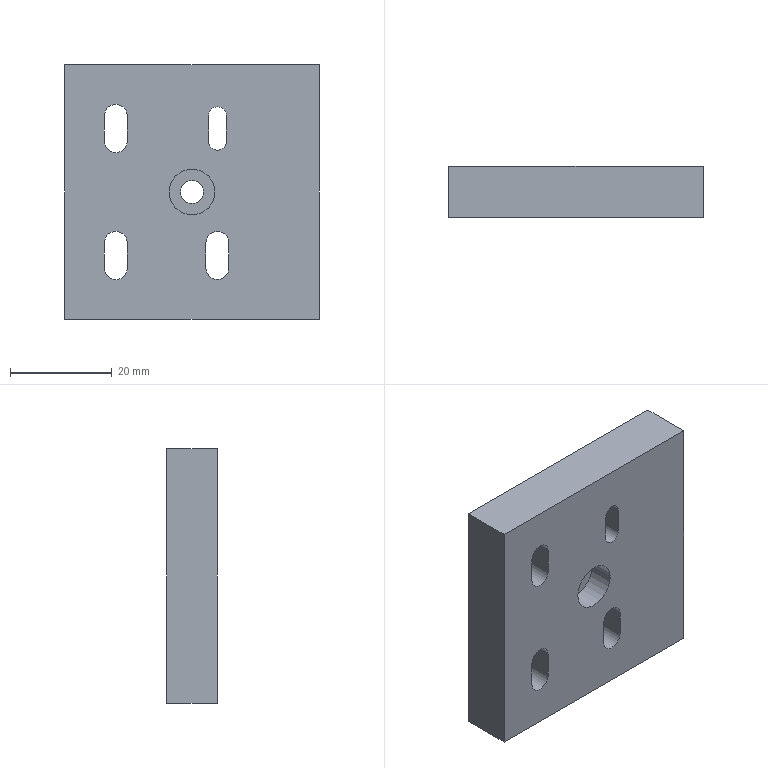Part | STEP file | 04-12 Guide cylinder base plate | 1 solid | 43 faces | box 50 x 10 x 50 mm | volume 22809 mm3 | cylinder 22 | plane 15 | cone 6 | commonest cylinder face diameters 4.5 x11 3.3 x6 3.5 x3 9 x2